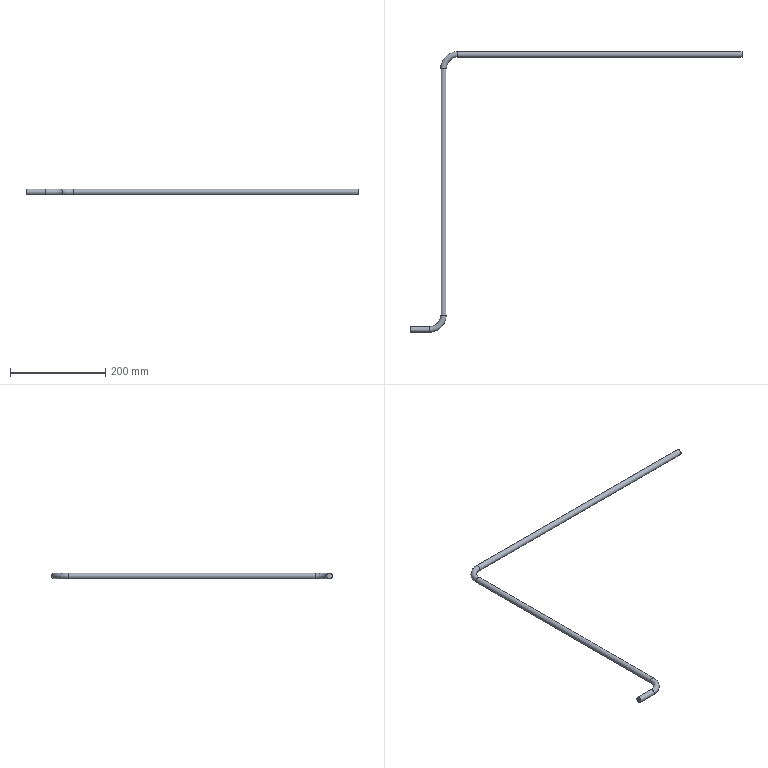Part | NX | features solid 2 | 1 solid | 7 faces | box 696 x 588.706 x 12 mm | volume 141027 mm3 | cylinder 3 | torus 2 | plane 2 | commonest cylinder face diameters 12 x3
STEP:
#1=CARTESIAN_POINT('',(860.,726.706,-496.));
#2=VERTEX_POINT('',#1);
#3=CARTESIAN_POINT('',(860.,726.706,-490.));
#4=DIRECTION('',(1.,0.,0.));
#5=DIRECTION('',(0.,0.,-1.));
#6=AXIS2_PLACEMENT_3D('',#3,#4,#5);
#7=CIRCLE('',#6,6.);
#8=EDGE_CURVE('',#2,#2,#7,.T.);
#9=ORIENTED_EDGE('',*,*,#8,.T.);
#10=EDGE_LOOP('',(#9));
#11=FACE_BOUND('',#10,.T.);
#12=CARTESIAN_POINT('',(1456.,726.706,-496.));
#13=VERTEX_POINT('',#12);
#14=CARTESIAN_POINT('',(1456.,726.706,-490.));
#15=DIRECTION('',(1.,0.,0.));
#16=DIRECTION('',(0.,0.,-1.));
#17=AXIS2_PLACEMENT_3D('',#14,#15,#16);
#18=CIRCLE('',#17,6.);
#19=EDGE_CURVE('',#13,#13,#18,.T.);
#20=ORIENTED_EDGE('',*,*,#19,.F.);
#21=EDGE_LOOP('',(#20));
#22=FACE_BOUND('',#21,.T.);
#23=CARTESIAN_POINT('',(860.,726.706,-490.));
#24=DIRECTION('',(1.,0.,0.));
#25=DIRECTION('',(0.,1.,0.));
#26=AXIS2_PLACEMENT_3D('',#23,#24,#25);
#27=CYLINDRICAL_SURFACE('',#26,6.);
#28=ADVANCED_FACE('',(#11,#22),#27,.T.);
#29=CARTESIAN_POINT('',(830.,696.706,-496.));
#30=VERTEX_POINT('',#29);
#31=CARTESIAN_POINT('',(830.,696.706,-490.));
#32=DIRECTION('',(0.,1.,0.));
#33=DIRECTION('',(0.,0.,-1.));
#34=AXIS2_PLACEMENT_3D('',#31,#32,#33);
#35=CIRCLE('',#34,6.);
#36=EDGE_CURVE('',#30,#30,#35,.T.);
#37=ORIENTED_EDGE('',*,*,#36,.T.);
#38=EDGE_LOOP('',(#37));
#39=FACE_BOUND('',#38,.T.);
#40=ORIENTED_EDGE('',*,*,#8,.F.);
#41=EDGE_LOOP('',(#40));
#42=FACE_BOUND('',#41,.T.);
#43=CARTESIAN_POINT('',(860.,696.706,-490.));
#44=DIRECTION('',(0.,0.,-1.));
#45=DIRECTION('',(-1.,0.,0.));
#46=AXIS2_PLACEMENT_3D('',#43,#44,#45);
#47=TOROIDAL_SURFACE('',#46,30.,6.);
#48=ADVANCED_FACE('',(#39,#42),#47,.T.);
#49=CARTESIAN_POINT('',(830.,180.,-496.));
#50=VERTEX_POINT('',#49);
#51=CARTESIAN_POINT('',(830.,180.,-490.));
#52=DIRECTION('',(0.,1.,0.));
#53=DIRECTION('',(0.,0.,-1.));
#54=AXIS2_PLACEMENT_3D('',#51,#52,#53);
#55=CIRCLE('',#54,6.);
#56=EDGE_CURVE('',#50,#50,#55,.T.);
#57=ORIENTED_EDGE('',*,*,#56,.T.);
#58=EDGE_LOOP('',(#57));
#59=FACE_BOUND('',#58,.T.);
#60=ORIENTED_EDGE('',*,*,#36,.F.);
#61=EDGE_LOOP('',(#60));
#62=FACE_BOUND('',#61,.T.);
#63=CARTESIAN_POINT('',(830.,180.,-490.));
#64=DIRECTION('',(0.,1.,0.));
#65=DIRECTION('',(0.,0.,1.));
#66=AXIS2_PLACEMENT_3D('',#63,#64,#65);
#67=CYLINDRICAL_SURFACE('',#66,6.);
#68=ADVANCED_FACE('',(#59,#62),#67,.T.);
#69=CARTESIAN_POINT('',(800.,150.,-496.));
#70=VERTEX_POINT('',#69);
#71=CARTESIAN_POINT('',(800.,150.,-490.));
#72=DIRECTION('',(1.,0.,0.));
#73=DIRECTION('',(0.,0.,-1.));
#74=AXIS2_PLACEMENT_3D('',#71,#72,#73);
#75=CIRCLE('',#74,6.);
#76=EDGE_CURVE('',#70,#70,#75,.T.);
#77=ORIENTED_EDGE('',*,*,#76,.T.);
#78=EDGE_LOOP('',(#77));
#79=FACE_BOUND('',#78,.T.);
#80=ORIENTED_EDGE('',*,*,#56,.F.);
#81=EDGE_LOOP('',(#80));
#82=FACE_BOUND('',#81,.T.);
#83=CARTESIAN_POINT('',(800.,180.,-490.));
#84=DIRECTION('',(0.,0.,1.));
#85=DIRECTION('',(1.,0.,0.));
#86=AXIS2_PLACEMENT_3D('',#83,#84,#85);
#87=TOROIDAL_SURFACE('',#86,30.,6.);
#88=ADVANCED_FACE('',(#79,#82),#87,.T.);
#89=ORIENTED_EDGE('',*,*,#76,.F.);
#90=EDGE_LOOP('',(#89));
#91=FACE_BOUND('',#90,.T.);
#92=CARTESIAN_POINT('',(760.,150.,-496.));
#93=VERTEX_POINT('',#92);
#94=CARTESIAN_POINT('',(760.,150.,-490.));
#95=DIRECTION('',(1.,0.,0.));
#96=DIRECTION('',(0.,0.,-1.));
#97=AXIS2_PLACEMENT_3D('',#94,#95,#96);
#98=CIRCLE('',#97,6.);
#99=EDGE_CURVE('',#93,#93,#98,.T.);
#100=ORIENTED_EDGE('',*,*,#99,.T.);
#101=EDGE_LOOP('',(#100));
#102=FACE_BOUND('',#101,.T.);
#103=CARTESIAN_POINT('',(800.,150.,-490.));
#104=DIRECTION('',(-1.,0.,0.));
#105=DIRECTION('',(0.,0.,1.));
#106=AXIS2_PLACEMENT_3D('',#103,#104,#105);
#107=CYLINDRICAL_SURFACE('',#106,6.);
#108=ADVANCED_FACE('',(#91,#102),#107,.T.);
#109=ORIENTED_EDGE('',*,*,#19,.T.);
#110=EDGE_LOOP('',(#109));
#111=FACE_BOUND('',#110,.T.);
#112=CARTESIAN_POINT('',(1456.,726.706,-490.));
#113=DIRECTION('',(1.,0.,0.));
#114=DIRECTION('',(0.,0.,-1.));
#115=AXIS2_PLACEMENT_3D('',#112,#113,#114);
#116=PLANE('',#115);
#117=ADVANCED_FACE('',(#111),#116,.T.);
#118=ORIENTED_EDGE('',*,*,#99,.F.);
#119=EDGE_LOOP('',(#118));
#120=FACE_BOUND('',#119,.T.);
#121=CARTESIAN_POINT('',(760.,150.,-490.));
#122=DIRECTION('',(1.,0.,0.));
#123=DIRECTION('',(0.,0.,-1.));
#124=AXIS2_PLACEMENT_3D('',#121,#122,#123);
#125=PLANE('',#124);
#126=ADVANCED_FACE('',(#120),#125,.F.);
#127=CLOSED_SHELL('',(#28,#48,#68,#88,#108,#117,#126));
#128=MANIFOLD_SOLID_BREP('',#127);
#129=(LENGTH_UNIT()NAMED_UNIT(*)SI_UNIT(.MILLI.,.METRE.));
#130=UNCERTAINTY_MEASURE_WITH_UNIT(LENGTH_MEASURE(0.00001),#129,'','');
#131=(NAMED_UNIT(*)PLANE_ANGLE_UNIT()SI_UNIT($,.RADIAN.));
#132=(NAMED_UNIT(*)SI_UNIT($,.STERADIAN.)SOLID_ANGLE_UNIT());
#133=(GEOMETRIC_REPRESENTATION_CONTEXT(3)GLOBAL_UNCERTAINTY_ASSIGNED_CONTEXT((#130))GLOBAL_UNIT_ASSIGNED_CONTEXT((#129,#131,#132))REPRESENTATION_CONTEXT('',''));
#134=ADVANCED_BREP_SHAPE_REPRESENTATION('',(#128),#133);